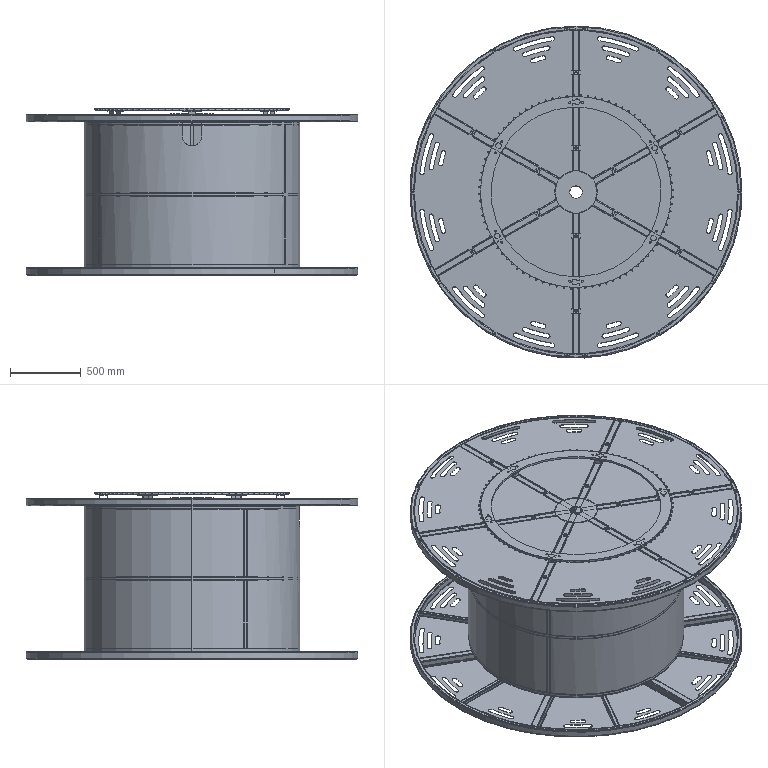Part | SolidWorks | features CompositeCurve 25, ReferencePattern 11, InContextFeatHolder 2, MirrorCompFeat 2, LocalCirPattern 1 | 65 solids | 4442 faces | volume 42347469 mm3 | cylinder 2239 | plane 1831 | torus 300 | cone 48 | spline 24 | commonest cylinder face diameters 6 x348 10 x204 22.306 x192 16.059 x174 41.467 x168 12 x104